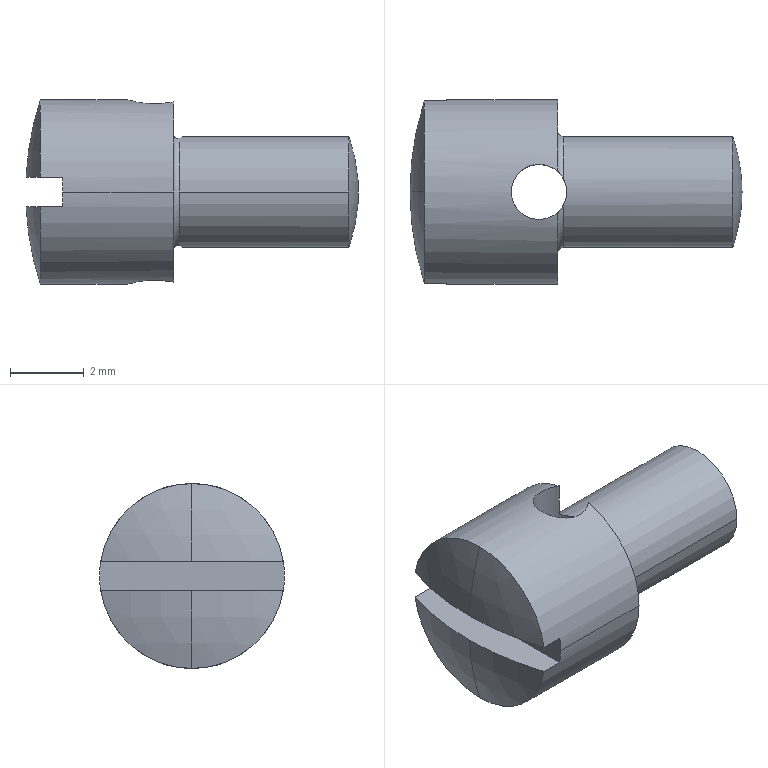Part | NX | features BREP 1 | 1 solid | 19 faces | box 8.99 x 5 x 5 mm | volume 97.359 mm3 | cylinder 6 | sphere 6 | plane 5 | torus 2 | commonest cylinder face diameters 1.5 x2 3 x2 5 x2
STEP:
#1=CARTESIAN_POINT('',(-3.,2.5,0.));
#2=VERTEX_POINT('',#1);
#3=CARTESIAN_POINT('',(0.,2.5,0.));
#4=VERTEX_POINT('',#3);
#5=CARTESIAN_POINT('',(-1.8,2.5,0.));
#6=DIRECTION('',(1.,0.,0.));
#7=VECTOR('',#6,1000.);
#8=LINE('',#5,#7);
#9=EDGE_CURVE('',#2,#4,#8,.T.);
#10=ORIENTED_EDGE('',*,*,#9,.F.);
#11=CARTESIAN_POINT('',(-3.,2.468,0.4));
#12=VERTEX_POINT('',#11);
#13=CARTESIAN_POINT('',(-3.,0.,0.));
#14=DIRECTION('',(1.,0.,0.));
#15=DIRECTION('',(0.,1.,0.));
#16=AXIS2_PLACEMENT_3D('',#13,#14,#15);
#17=CIRCLE('',#16,2.5);
#18=EDGE_CURVE('',#2,#12,#17,.T.);
#19=ORIENTED_EDGE('',*,*,#18,.T.);
#20=CARTESIAN_POINT('',(-3.599,2.468,0.4));
#21=VERTEX_POINT('',#20);
#22=CARTESIAN_POINT('',(-3.3,2.468,0.4));
#23=DIRECTION('',(-1.,0.,0.));
#24=VECTOR('',#23,1000.);
#25=LINE('',#22,#24);
#26=EDGE_CURVE('',#12,#21,#25,.T.);
#27=ORIENTED_EDGE('',*,*,#26,.T.);
#28=CARTESIAN_POINT('',(-3.599,0.,2.5));
#29=VERTEX_POINT('',#28);
#30=CARTESIAN_POINT('',(-3.599,0.,0.));
#31=DIRECTION('',(1.,0.,0.));
#32=DIRECTION('',(0.,1.,0.));
#33=AXIS2_PLACEMENT_3D('',#30,#31,#32);
#34=CIRCLE('',#33,2.5);
#35=EDGE_CURVE('',#21,#29,#34,.T.);
#36=ORIENTED_EDGE('',*,*,#35,.T.);
#37=CARTESIAN_POINT('',(-3.599,-2.468,0.4));
#38=VERTEX_POINT('',#37);
#39=CARTESIAN_POINT('',(-3.599,0.,0.));
#40=DIRECTION('',(1.,0.,0.));
#41=DIRECTION('',(0.,1.,0.));
#42=AXIS2_PLACEMENT_3D('',#39,#40,#41);
#43=CIRCLE('',#42,2.5);
#44=EDGE_CURVE('',#29,#38,#43,.T.);
#45=ORIENTED_EDGE('',*,*,#44,.T.);
#46=CARTESIAN_POINT('',(-3.,-2.468,0.4));
#47=VERTEX_POINT('',#46);
#48=CARTESIAN_POINT('',(-3.3,-2.468,0.4));
#49=DIRECTION('',(1.,0.,0.));
#50=VECTOR('',#49,1000.);
#51=LINE('',#48,#50);
#52=EDGE_CURVE('',#38,#47,#51,.T.);
#53=ORIENTED_EDGE('',*,*,#52,.T.);
#54=CARTESIAN_POINT('',(-3.,-2.5,0.));
#55=VERTEX_POINT('',#54);
#56=CARTESIAN_POINT('',(-3.,0.,0.));
#57=DIRECTION('',(1.,0.,0.));
#58=DIRECTION('',(0.,1.,0.));
#59=AXIS2_PLACEMENT_3D('',#56,#57,#58);
#60=CIRCLE('',#59,2.5);
#61=EDGE_CURVE('',#47,#55,#60,.T.);
#62=ORIENTED_EDGE('',*,*,#61,.T.);
#63=CARTESIAN_POINT('',(0.,-2.5,0.));
#64=VERTEX_POINT('',#63);
#65=CARTESIAN_POINT('',(-1.8,-2.5,0.));
#66=DIRECTION('',(-1.,0.,0.));
#67=VECTOR('',#66,1000.);
#68=LINE('',#65,#67);
#69=EDGE_CURVE('',#64,#55,#68,.T.);
#70=ORIENTED_EDGE('',*,*,#69,.F.);
#71=CARTESIAN_POINT('',(0.,-0.559,2.437));
#72=VERTEX_POINT('',#71);
#73=CARTESIAN_POINT('',(0.,0.,0.));
#74=DIRECTION('',(1.,0.,0.));
#75=DIRECTION('',(0.,1.,0.));
#76=AXIS2_PLACEMENT_3D('',#73,#74,#75);
#77=CIRCLE('',#76,2.5);
#78=EDGE_CURVE('',#72,#64,#77,.T.);
#79=ORIENTED_EDGE('',*,*,#78,.F.);
#80=CARTESIAN_POINT('',(-1.25,0.,2.5));
#81=VERTEX_POINT('',#80);
#82=CARTESIAN_POINT('',(0.,-0.559,2.437));
#83=CARTESIAN_POINT('',(-0.215,-0.7513,2.393));
#84=CARTESIAN_POINT('',(-0.8817,-0.8468,2.363));
#85=CARTESIAN_POINT('',(-1.25,-0.2921,2.5));
#86=CARTESIAN_POINT('',(-1.25,0.,2.5));
#87=B_SPLINE_CURVE_WITH_KNOTS('',3,(#82,#83,#84,#85,#86),.UNSPECIFIED.,.F.,.F.,(4,1,4),(0.,0.0008635,0.001727),.UNSPECIFIED.);
#88=EDGE_CURVE('',#72,#81,#87,.T.);
#89=ORIENTED_EDGE('',*,*,#88,.T.);
#90=CARTESIAN_POINT('',(0.,0.559,2.437));
#91=VERTEX_POINT('',#90);
#92=CARTESIAN_POINT('',(-1.25,0.,2.5));
#93=CARTESIAN_POINT('',(-1.25,0.292,2.5));
#94=CARTESIAN_POINT('',(-0.882,0.8466,2.363));
#95=CARTESIAN_POINT('',(-0.2151,0.7514,2.393));
#96=CARTESIAN_POINT('',(0.,0.559,2.437));
#97=B_SPLINE_CURVE_WITH_KNOTS('',3,(#92,#93,#94,#95,#96),.UNSPECIFIED.,.F.,.F.,(4,1,4),(0.,0.0008633,0.001727),.UNSPECIFIED.);
#98=EDGE_CURVE('',#81,#91,#97,.T.);
#99=ORIENTED_EDGE('',*,*,#98,.T.);
#100=CARTESIAN_POINT('',(0.,0.,0.));
#101=DIRECTION('',(1.,0.,0.));
#102=DIRECTION('',(0.,1.,0.));
#103=AXIS2_PLACEMENT_3D('',#100,#101,#102);
#104=CIRCLE('',#103,2.5);
#105=EDGE_CURVE('',#4,#91,#104,.T.);
#106=ORIENTED_EDGE('',*,*,#105,.F.);
#107=EDGE_LOOP('',(#10,#19,#27,#36,#45,#53,#62,#70,#79,#89,#99,#106));
#108=FACE_BOUND('',#107,.T.);
#109=CARTESIAN_POINT('',(-1.8,0.,0.));
#110=DIRECTION('',(1.,0.,0.));
#111=DIRECTION('',(0.,-1.,0.));
#112=AXIS2_PLACEMENT_3D('',#109,#110,#111);
#113=CYLINDRICAL_SURFACE('',#112,2.5);
#114=ADVANCED_FACE('',(#108),#113,.T.);
#115=CARTESIAN_POINT('',(4.743,0.,-1.5));
#116=VERTEX_POINT('',#115);
#117=CARTESIAN_POINT('',(4.743,0.,1.5));
#118=VERTEX_POINT('',#117);
#119=CARTESIAN_POINT('',(0.5,0.,0.));
#120=DIRECTION('',(0.,-1.,0.));
#121=DIRECTION('',(0.,0.,1.));
#122=AXIS2_PLACEMENT_3D('',#119,#120,#121);
#123=CIRCLE('',#122,4.5);
#124=EDGE_CURVE('',#116,#118,#123,.T.);
#125=ORIENTED_EDGE('',*,*,#124,.F.);
#126=CARTESIAN_POINT('',(4.743,1.5,0.));
#127=VERTEX_POINT('',#126);
#128=CARTESIAN_POINT('',(4.743,0.,0.));
#129=DIRECTION('',(1.,0.,0.));
#130=DIRECTION('',(0.,1.,0.));
#131=AXIS2_PLACEMENT_3D('',#128,#129,#130);
#132=CIRCLE('',#131,1.5);
#133=EDGE_CURVE('',#116,#127,#132,.T.);
#134=ORIENTED_EDGE('',*,*,#133,.T.);
#135=CARTESIAN_POINT('',(4.743,0.,0.));
#136=DIRECTION('',(1.,0.,0.));
#137=DIRECTION('',(0.,1.,0.));
#138=AXIS2_PLACEMENT_3D('',#135,#136,#137);
#139=CIRCLE('',#138,1.5);
#140=EDGE_CURVE('',#127,#118,#139,.T.);
#141=ORIENTED_EDGE('',*,*,#140,.T.);
#142=EDGE_LOOP('',(#125,#134,#141));
#143=FACE_BOUND('',#142,.T.);
#144=CARTESIAN_POINT('',(0.5,0.,0.));
#145=DIRECTION('',(0.,0.,1.));
#146=DIRECTION('',(-1.,0.,0.));
#147=AXIS2_PLACEMENT_3D('',#144,#145,#146);
#148=SPHERICAL_SURFACE('',#147,4.5);
#149=ADVANCED_FACE('',(#143),#148,.T.);
#150=CARTESIAN_POINT('',(-3.99,0.,0.4));
#151=VERTEX_POINT('',#150);
#152=CARTESIAN_POINT('',(4.,0.,0.));
#153=DIRECTION('',(0.,-1.,0.));
#154=DIRECTION('',(0.,0.,1.));
#155=AXIS2_PLACEMENT_3D('',#152,#153,#154);
#156=CIRCLE('',#155,8.);
#157=EDGE_CURVE('',#29,#151,#156,.T.);
#158=ORIENTED_EDGE('',*,*,#157,.F.);
#159=ORIENTED_EDGE('',*,*,#35,.F.);
#160=CARTESIAN_POINT('',(4.,0.,0.4));
#161=DIRECTION('',(0.,0.,1.));
#162=DIRECTION('',(0.,1.,0.));
#163=AXIS2_PLACEMENT_3D('',#160,#161,#162);
#164=CIRCLE('',#163,7.99);
#165=EDGE_CURVE('',#21,#151,#164,.T.);
#166=ORIENTED_EDGE('',*,*,#165,.T.);
#167=EDGE_LOOP('',(#158,#159,#166));
#168=FACE_BOUND('',#167,.T.);
#169=CARTESIAN_POINT('',(4.,0.,0.));
#170=DIRECTION('',(0.,0.,1.));
#171=DIRECTION('',(-1.,0.,0.));
#172=AXIS2_PLACEMENT_3D('',#169,#170,#171);
#173=SPHERICAL_SURFACE('',#172,8.);
#174=ADVANCED_FACE('',(#168),#173,.T.);
#175=CARTESIAN_POINT('',(-3.99,0.,-0.4));
#176=VERTEX_POINT('',#175);
#177=CARTESIAN_POINT('',(-3.599,0.,-2.5));
#178=VERTEX_POINT('',#177);
#179=CARTESIAN_POINT('',(4.,0.,0.));
#180=DIRECTION('',(0.,-1.,0.));
#181=DIRECTION('',(0.,0.,1.));
#182=AXIS2_PLACEMENT_3D('',#179,#180,#181);
#183=CIRCLE('',#182,8.);
#184=EDGE_CURVE('',#176,#178,#183,.T.);
#185=ORIENTED_EDGE('',*,*,#184,.F.);
#186=CARTESIAN_POINT('',(-3.599,2.468,-0.4));
#187=VERTEX_POINT('',#186);
#188=CARTESIAN_POINT('',(4.,0.,-0.4));
#189=DIRECTION('',(0.,0.,-1.));
#190=DIRECTION('',(0.,-1.,0.));
#191=AXIS2_PLACEMENT_3D('',#188,#189,#190);
#192=CIRCLE('',#191,7.99);
#193=EDGE_CURVE('',#176,#187,#192,.T.);
#194=ORIENTED_EDGE('',*,*,#193,.T.);
#195=CARTESIAN_POINT('',(-3.599,0.,0.));
#196=DIRECTION('',(1.,0.,0.));
#197=DIRECTION('',(0.,1.,0.));
#198=AXIS2_PLACEMENT_3D('',#195,#196,#197);
#199=CIRCLE('',#198,2.5);
#200=EDGE_CURVE('',#178,#187,#199,.T.);
#201=ORIENTED_EDGE('',*,*,#200,.F.);
#202=EDGE_LOOP('',(#185,#194,#201));
#203=FACE_BOUND('',#202,.T.);
#204=CARTESIAN_POINT('',(4.,0.,0.));
#205=DIRECTION('',(0.,0.,1.));
#206=DIRECTION('',(-1.,0.,0.));
#207=AXIS2_PLACEMENT_3D('',#204,#205,#206);
#208=SPHERICAL_SURFACE('',#207,8.);
#209=ADVANCED_FACE('',(#203),#208,.T.);
#210=CARTESIAN_POINT('',(0.1624,1.5,0.));
#211=VERTEX_POINT('',#210);
#212=CARTESIAN_POINT('',(2.453,1.5,0.));
#213=DIRECTION('',(1.,0.,0.));
#214=VECTOR('',#213,1000.);
#215=LINE('',#212,#214);
#216=EDGE_CURVE('',#211,#127,#215,.T.);
#217=ORIENTED_EDGE('',*,*,#216,.F.);
#218=CARTESIAN_POINT('',(0.1624,0.3518,1.458));
#219=VERTEX_POINT('',#218);
#220=CARTESIAN_POINT('',(0.1624,0.,0.));
#221=DIRECTION('',(1.,0.,0.));
#222=DIRECTION('',(0.,1.,0.));
#223=AXIS2_PLACEMENT_3D('',#220,#221,#222);
#224=CIRCLE('',#223,1.5);
#225=EDGE_CURVE('',#211,#219,#224,.T.);
#226=ORIENTED_EDGE('',*,*,#225,.T.);
#227=CARTESIAN_POINT('',(0.25,0.,1.5));
#228=VERTEX_POINT('',#227);
#229=CARTESIAN_POINT('',(0.1624,0.3518,1.458));
#230=CARTESIAN_POINT('',(0.2192,0.2448,1.484));
#231=CARTESIAN_POINT('',(0.25,0.124,1.5));
#232=CARTESIAN_POINT('',(0.25,0.,1.5));
#233=B_SPLINE_CURVE_WITH_KNOTS('',3,(#229,#230,#231,#232),.UNSPECIFIED.,.F.,.F.,(4,4),(0.,0.0003667),.UNSPECIFIED.);
#234=EDGE_CURVE('',#219,#228,#233,.T.);
#235=ORIENTED_EDGE('',*,*,#234,.T.);
#236=CARTESIAN_POINT('',(0.1624,-0.3518,1.458));
#237=VERTEX_POINT('',#236);
#238=CARTESIAN_POINT('',(0.25,0.,1.5));
#239=CARTESIAN_POINT('',(0.25,-0.124,1.5));
#240=CARTESIAN_POINT('',(0.2192,-0.2447,1.484));
#241=CARTESIAN_POINT('',(0.1624,-0.3518,1.458));
#242=B_SPLINE_CURVE_WITH_KNOTS('',3,(#238,#239,#240,#241),.UNSPECIFIED.,.F.,.F.,(4,4),(0.,0.0003665),.UNSPECIFIED.);
#243=EDGE_CURVE('',#228,#237,#242,.T.);
#244=ORIENTED_EDGE('',*,*,#243,.T.);
#245=CARTESIAN_POINT('',(0.1624,-1.5,0.));
#246=VERTEX_POINT('',#245);
#247=CARTESIAN_POINT('',(0.1624,0.,0.));
#248=DIRECTION('',(1.,0.,0.));
#249=DIRECTION('',(0.,1.,0.));
#250=AXIS2_PLACEMENT_3D('',#247,#248,#249);
#251=CIRCLE('',#250,1.5);
#252=EDGE_CURVE('',#237,#246,#251,.T.);
#253=ORIENTED_EDGE('',*,*,#252,.T.);
#254=CARTESIAN_POINT('',(4.743,-1.5,0.));
#255=VERTEX_POINT('',#254);
#256=CARTESIAN_POINT('',(2.453,-1.5,0.));
#257=DIRECTION('',(-1.,0.,0.));
#258=VECTOR('',#257,1000.);
#259=LINE('',#256,#258);
#260=EDGE_CURVE('',#255,#246,#259,.T.);
#261=ORIENTED_EDGE('',*,*,#260,.F.);
#262=CARTESIAN_POINT('',(4.743,0.,0.));
#263=DIRECTION('',(1.,0.,0.));
#264=DIRECTION('',(0.,1.,0.));
#265=AXIS2_PLACEMENT_3D('',#262,#263,#264);
#266=CIRCLE('',#265,1.5);
#267=EDGE_CURVE('',#118,#255,#266,.T.);
#268=ORIENTED_EDGE('',*,*,#267,.F.);
#269=ORIENTED_EDGE('',*,*,#140,.F.);
#270=EDGE_LOOP('',(#217,#226,#235,#244,#253,#261,#268,#269));
#271=FACE_BOUND('',#270,.T.);
#272=CARTESIAN_POINT('',(2.453,0.,0.));
#273=DIRECTION('',(1.,0.,0.));
#274=DIRECTION('',(0.,-1.,0.));
#275=AXIS2_PLACEMENT_3D('',#272,#273,#274);
#276=CYLINDRICAL_SURFACE('',#275,1.5);
#277=ADVANCED_FACE('',(#271),#276,.T.);
#278=CARTESIAN_POINT('',(0.25,0.,-1.5));
#279=VERTEX_POINT('',#278);
#280=CARTESIAN_POINT('',(0.25,0.,0.));
#281=DIRECTION('',(0.,0.,-1.));
#282=VECTOR('',#281,1000.);
#283=LINE('',#280,#282);
#284=EDGE_CURVE('',#228,#279,#283,.T.);
#285=ORIENTED_EDGE('',*,*,#284,.F.);
#286=ORIENTED_EDGE('',*,*,#234,.F.);
#287=CARTESIAN_POINT('',(0.,0.559,1.566));
#288=VERTEX_POINT('',#287);
#289=CARTESIAN_POINT('',(0.,0.559,1.566));
#290=CARTESIAN_POINT('',(0.,0.559,1.453));
#291=CARTESIAN_POINT('',(0.1113,0.4479,1.435));
#292=CARTESIAN_POINT('',(0.1624,0.3518,1.458));
#293=B_SPLINE_CURVE_WITH_KNOTS('',3,(#289,#290,#291,#292),.UNSPECIFIED.,.F.,.F.,(4,4),(0.,0.0003331),.UNSPECIFIED.);
#294=EDGE_CURVE('',#288,#219,#293,.T.);
#295=ORIENTED_EDGE('',*,*,#294,.F.);
#296=CARTESIAN_POINT('',(0.,0.559,0.));
#297=DIRECTION('',(0.,0.,-1.));
#298=VECTOR('',#297,1000.);
#299=LINE('',#296,#298);
#300=EDGE_CURVE('',#91,#288,#299,.T.);
#301=ORIENTED_EDGE('',*,*,#300,.F.);
#302=ORIENTED_EDGE('',*,*,#98,.F.);
#303=CARTESIAN_POINT('',(-1.25,0.,-2.5));
#304=VERTEX_POINT('',#303);
#305=CARTESIAN_POINT('',(-1.25,0.,0.));
#306=DIRECTION('',(0.,0.,1.));
#307=VECTOR('',#306,1000.);
#308=LINE('',#305,#307);
#309=EDGE_CURVE('',#304,#81,#308,.T.);
#310=ORIENTED_EDGE('',*,*,#309,.F.);
#311=CARTESIAN_POINT('',(0.,0.559,-2.437));
#312=VERTEX_POINT('',#311);
#313=CARTESIAN_POINT('',(0.,0.559,-2.437));
#314=CARTESIAN_POINT('',(-0.215,0.7513,-2.393));
#315=CARTESIAN_POINT('',(-0.8817,0.8468,-2.363));
#316=CARTESIAN_POINT('',(-1.25,0.2921,-2.5));
#317=CARTESIAN_POINT('',(-1.25,0.,-2.5));
#318=B_SPLINE_CURVE_WITH_KNOTS('',3,(#313,#314,#315,#316,#317),.UNSPECIFIED.,.F.,.F.,(4,1,4),(0.,0.0008635,0.001727),.UNSPECIFIED.);
#319=EDGE_CURVE('',#312,#304,#318,.T.);
#320=ORIENTED_EDGE('',*,*,#319,.F.);
#321=CARTESIAN_POINT('',(0.,0.559,-1.566));
#322=VERTEX_POINT('',#321);
#323=CARTESIAN_POINT('',(0.,0.559,0.));
#324=DIRECTION('',(0.,0.,-1.));
#325=VECTOR('',#324,1000.);
#326=LINE('',#323,#325);
#327=EDGE_CURVE('',#322,#312,#326,.T.);
#328=ORIENTED_EDGE('',*,*,#327,.F.);
#329=CARTESIAN_POINT('',(0.1624,0.3518,-1.458));
#330=VERTEX_POINT('',#329);
#331=CARTESIAN_POINT('',(0.1624,0.3518,-1.458));
#332=CARTESIAN_POINT('',(0.1464,0.3819,-1.451));
#333=CARTESIAN_POINT('',(0.1296,0.4086,-1.446));
#334=CARTESIAN_POINT('',(0.0958,0.4565,-1.443));
#335=CARTESIAN_POINT('',(0.07987,0.4762,-1.445));
#336=CARTESIAN_POINT('',(0.055,0.5047,-1.455));
#337=CARTESIAN_POINT('',(0.04446,0.516,-1.461));
#338=CARTESIAN_POINT('',(0.02656,0.5342,-1.479));
#339=CARTESIAN_POINT('',(0.01932,0.5412,-1.489));
#340=CARTESIAN_POINT('',(0.007644,0.5521,-1.513));
#341=CARTESIAN_POINT('',(0.003645,0.5557,-1.527));
#342=CARTESIAN_POINT('',(-0.0008785,0.5598,-1.56));
#343=CARTESIAN_POINT('',(-0.0003757,0.5594,-1.578));
#344=CARTESIAN_POINT('',(0.005894,0.5537,-1.618));
#345=CARTESIAN_POINT('',(0.01314,0.5472,-1.641));
#346=CARTESIAN_POINT('',(0.02374,0.5368,-1.662));
#347=B_SPLINE_CURVE_WITH_KNOTS('',3,(#331,#332,#333,#334,#335,#336,#337,#338,#339,#340,#341,#342,#343,#344,#345,#346),.UNSPECIFIED.,.F.,.F.,(4,2,2,2,2,2,2,4),(0.,0.169,0.3392,0.466,0.5754,0.6889,0.8273,1.),.UNSPECIFIED.);
#348=EDGE_CURVE('',#330,#322,#347,.T.);
#349=ORIENTED_EDGE('',*,*,#348,.F.);
#350=CARTESIAN_POINT('',(0.25,0.,-1.5));
#351=CARTESIAN_POINT('',(0.25,0.124,-1.5));
#352=CARTESIAN_POINT('',(0.2192,0.2447,-1.484));
#353=CARTESIAN_POINT('',(0.1624,0.3518,-1.458));
#354=B_SPLINE_CURVE_WITH_KNOTS('',3,(#350,#351,#352,#353),.UNSPECIFIED.,.F.,.F.,(4,4),(0.,0.0003665),.UNSPECIFIED.);
#355=EDGE_CURVE('',#279,#330,#354,.T.);
#356=ORIENTED_EDGE('',*,*,#355,.F.);
#357=EDGE_LOOP('',(#285,#286,#295,#301,#302,#310,#320,#328,#349,#356));
#358=FACE_BOUND('',#357,.T.);
#359=CARTESIAN_POINT('',(-0.5,0.,0.));
#360=DIRECTION('',(0.,0.,1.));
#361=DIRECTION('',(-1.,0.,0.));
#362=AXIS2_PLACEMENT_3D('',#359,#360,#361);
#363=CYLINDRICAL_SURFACE('',#362,0.75);
#364=ADVANCED_FACE('',(#358),#363,.F.);
#365=ORIENTED_EDGE('',*,*,#284,.T.);
#366=CARTESIAN_POINT('',(0.1624,-0.3518,-1.458));
#367=VERTEX_POINT('',#366);
#368=CARTESIAN_POINT('',(0.1624,-0.3518,-1.458));
#369=CARTESIAN_POINT('',(0.2192,-0.2448,-1.484));
#370=CARTESIAN_POINT('',(0.25,-0.124,-1.5));
#371=CARTESIAN_POINT('',(0.25,0.,-1.5));
#372=B_SPLINE_CURVE_WITH_KNOTS('',3,(#368,#369,#370,#371),.UNSPECIFIED.,.F.,.F.,(4,4),(0.,0.0003667),.UNSPECIFIED.);
#373=EDGE_CURVE('',#367,#279,#372,.T.);
#374=ORIENTED_EDGE('',*,*,#373,.F.);
#375=CARTESIAN_POINT('',(0.,-0.559,-1.566));
#376=VERTEX_POINT('',#375);
#377=CARTESIAN_POINT('',(0.,-0.559,-1.566));
#378=CARTESIAN_POINT('',(0.,-0.559,-1.453));
#379=CARTESIAN_POINT('',(0.1113,-0.4479,-1.435));
#380=CARTESIAN_POINT('',(0.1624,-0.3518,-1.458));
#381=B_SPLINE_CURVE_WITH_KNOTS('',3,(#377,#378,#379,#380),.UNSPECIFIED.,.F.,.F.,(4,4),(0.,0.0003331),.UNSPECIFIED.);
#382=EDGE_CURVE('',#376,#367,#381,.T.);
#383=ORIENTED_EDGE('',*,*,#382,.F.);
#384=CARTESIAN_POINT('',(0.,-0.559,-2.437));
#385=VERTEX_POINT('',#384);
#386=CARTESIAN_POINT('',(0.,-0.559,0.));
#387=DIRECTION('',(0.,0.,1.));
#388=VECTOR('',#387,1000.);
#389=LINE('',#386,#388);
#390=EDGE_CURVE('',#385,#376,#389,.T.);
#391=ORIENTED_EDGE('',*,*,#390,.F.);
#392=CARTESIAN_POINT('',(-1.25,0.,-2.5));
#393=CARTESIAN_POINT('',(-1.25,-0.292,-2.5));
#394=CARTESIAN_POINT('',(-0.882,-0.8466,-2.363));
#395=CARTESIAN_POINT('',(-0.2151,-0.7514,-2.393));
#396=CARTESIAN_POINT('',(0.,-0.559,-2.437));
#397=B_SPLINE_CURVE_WITH_KNOTS('',3,(#392,#393,#394,#395,#396),.UNSPECIFIED.,.F.,.F.,(4,1,4),(0.,0.0008633,0.001727),.UNSPECIFIED.);
#398=EDGE_CURVE('',#304,#385,#397,.T.);
#399=ORIENTED_EDGE('',*,*,#398,.F.);
#400=ORIENTED_EDGE('',*,*,#309,.T.);
#401=ORIENTED_EDGE('',*,*,#88,.F.);
#402=CARTESIAN_POINT('',(0.,-0.559,1.566));
#403=VERTEX_POINT('',#402);
#404=CARTESIAN_POINT('',(0.,-0.559,0.));
#405=DIRECTION('',(0.,0.,1.));
#406=VECTOR('',#405,1000.);
#407=LINE('',#404,#406);
#408=EDGE_CURVE('',#403,#72,#407,.T.);
#409=ORIENTED_EDGE('',*,*,#408,.F.);
#410=CARTESIAN_POINT('',(0.1624,-0.3518,1.458));
#411=CARTESIAN_POINT('',(0.1464,-0.3819,1.451));
#412=CARTESIAN_POINT('',(0.1296,-0.4086,1.446));
#413=CARTESIAN_POINT('',(0.0958,-0.4565,1.443));
#414=CARTESIAN_POINT('',(0.07987,-0.4762,1.445));
#415=CARTESIAN_POINT('',(0.055,-0.5047,1.455));
#416=CARTESIAN_POINT('',(0.04446,-0.516,1.461));
#417=CARTESIAN_POINT('',(0.02656,-0.5342,1.479));
#418=CARTESIAN_POINT('',(0.01932,-0.5412,1.489));
#419=CARTESIAN_POINT('',(0.007644,-0.5521,1.513));
#420=CARTESIAN_POINT('',(0.003645,-0.5557,1.527));
#421=CARTESIAN_POINT('',(-0.0008785,-0.5598,1.56));
#422=CARTESIAN_POINT('',(-0.0003757,-0.5594,1.578));
#423=CARTESIAN_POINT('',(0.005894,-0.5537,1.618));
#424=CARTESIAN_POINT('',(0.01314,-0.5472,1.641));
#425=CARTESIAN_POINT('',(0.02374,-0.5368,1.662));
#426=B_SPLINE_CURVE_WITH_KNOTS('',3,(#410,#411,#412,#413,#414,#415,#416,#417,#418,#419,#420,#421,#422,#423,#424,#425),.UNSPECIFIED.,.F.,.F.,(4,2,2,2,2,2,2,4),(0.,0.169,0.3392,0.466,0.5754,0.6889,0.8273,1.),.UNSPECIFIED.);
#427=EDGE_CURVE('',#237,#403,#426,.T.);
#428=ORIENTED_EDGE('',*,*,#427,.F.);
#429=ORIENTED_EDGE('',*,*,#243,.F.);
#430=EDGE_LOOP('',(#365,#374,#383,#391,#399,#400,#401,#409,#428,#429));
#431=FACE_BOUND('',#430,.T.);
#432=CARTESIAN_POINT('',(-0.5,0.,0.));
#433=DIRECTION('',(0.,0.,1.));
#434=DIRECTION('',(-1.,0.,0.));
#435=AXIS2_PLACEMENT_3D('',#432,#433,#434);
#436=CYLINDRICAL_SURFACE('',#435,0.75);
#437=ADVANCED_FACE('',(#431),#436,.F.);
#438=ORIENTED_EDGE('',*,*,#216,.T.);
#439=ORIENTED_EDGE('',*,*,#133,.F.);
#440=CARTESIAN_POINT('',(4.743,0.,0.));
#441=DIRECTION('',(1.,0.,0.));
#442=DIRECTION('',(0.,1.,0.));
#443=AXIS2_PLACEMENT_3D('',#440,#441,#442);
#444=CIRCLE('',#443,1.5);
#445=EDGE_CURVE('',#255,#116,#444,.T.);
#446=ORIENTED_EDGE('',*,*,#445,.F.);
#447=ORIENTED_EDGE('',*,*,#260,.T.);
#448=CARTESIAN_POINT('',(0.1624,0.,0.));
#449=DIRECTION('',(1.,0.,0.));
#450=DIRECTION('',(0.,1.,0.));
#451=AXIS2_PLACEMENT_3D('',#448,#449,#450);
#452=CIRCLE('',#451,1.5);
#453=EDGE_CURVE('',#246,#367,#452,.T.);
#454=ORIENTED_EDGE('',*,*,#453,.T.);
#455=ORIENTED_EDGE('',*,*,#373,.T.);
#456=ORIENTED_EDGE('',*,*,#355,.T.);
#457=CARTESIAN_POINT('',(0.1624,0.,0.));
#458=DIRECTION('',(1.,0.,0.));
#459=DIRECTION('',(0.,1.,0.));
#460=AXIS2_PLACEMENT_3D('',#457,#458,#459);
#461=CIRCLE('',#460,1.5);
#462=EDGE_CURVE('',#330,#211,#461,.T.);
#463=ORIENTED_EDGE('',*,*,#462,.T.);
#464=EDGE_LOOP('',(#438,#439,#446,#447,#454,#455,#456,#463));
#465=FACE_BOUND('',#464,.T.);
#466=CARTESIAN_POINT('',(2.453,0.,0.));
#467=DIRECTION('',(1.,0.,0.));
#468=DIRECTION('',(0.,-1.,0.));
#469=AXIS2_PLACEMENT_3D('',#466,#467,#468);
#470=CYLINDRICAL_SURFACE('',#469,1.5);
#471=ADVANCED_FACE('',(#465),#470,.T.);
#472=ORIENTED_EDGE('',*,*,#427,.T.);
#473=CARTESIAN_POINT('',(0.,0.,0.));
#474=DIRECTION('',(1.,0.,0.));
#475=DIRECTION('',(0.,1.,0.));
#476=AXIS2_PLACEMENT_3D('',#473,#474,#475);
#477=CIRCLE('',#476,1.662);
#478=EDGE_CURVE('',#403,#376,#477,.T.);
#479=ORIENTED_EDGE('',*,*,#478,.T.);
#480=ORIENTED_EDGE('',*,*,#382,.T.);
#481=ORIENTED_EDGE('',*,*,#453,.F.);
#482=ORIENTED_EDGE('',*,*,#252,.F.);
#483=EDGE_LOOP('',(#472,#479,#480,#481,#482));
#484=FACE_BOUND('',#483,.T.);
#485=CARTESIAN_POINT('',(0.1624,0.,0.));
#486=DIRECTION('',(1.,0.,0.));
#487=DIRECTION('',(0.,0.,1.));
#488=AXIS2_PLACEMENT_3D('',#485,#486,#487);
#489=TOROIDAL_SURFACE('',#488,1.662,0.1624);
#490=ADVANCED_FACE('',(#484),#489,.F.);
#491=ORIENTED_EDGE('',*,*,#408,.T.);
#492=ORIENTED_EDGE('',*,*,#78,.T.);
#493=CARTESIAN_POINT('',(0.,0.,0.));
#494=DIRECTION('',(1.,0.,0.));
#495=DIRECTION('',(0.,1.,0.));
#496=AXIS2_PLACEMENT_3D('',#493,#494,#495);
#497=CIRCLE('',#496,2.5);
#498=EDGE_CURVE('',#64,#385,#497,.T.);
#499=ORIENTED_EDGE('',*,*,#498,.T.);
#500=ORIENTED_EDGE('',*,*,#390,.T.);
#501=ORIENTED_EDGE('',*,*,#478,.F.);
#502=EDGE_LOOP('',(#491,#492,#499,#500,#501));
#503=FACE_BOUND('',#502,.T.);
#504=CARTESIAN_POINT('',(0.,2.081,0.));
#505=DIRECTION('',(1.,0.,0.));
#506=DIRECTION('',(0.,-1.,0.));
#507=AXIS2_PLACEMENT_3D('',#504,#505,#506);
#508=PLANE('',#507);
#509=ADVANCED_FACE('',(#503),#508,.T.);
#510=ORIENTED_EDGE('',*,*,#26,.F.);
#511=CARTESIAN_POINT('',(-3.,0.,0.4));
#512=DIRECTION('',(0.,1.,0.));
#513=VECTOR('',#512,1000.);
#514=LINE('',#511,#513);
#515=EDGE_CURVE('',#47,#12,#514,.T.);
#516=ORIENTED_EDGE('',*,*,#515,.F.);
#517=ORIENTED_EDGE('',*,*,#52,.F.);
#518=CARTESIAN_POINT('',(4.,0.,0.4));
#519=DIRECTION('',(0.,0.,1.));
#520=DIRECTION('',(0.,1.,0.));
#521=AXIS2_PLACEMENT_3D('',#518,#519,#520);
#522=CIRCLE('',#521,7.99);
#523=EDGE_CURVE('',#151,#38,#522,.T.);
#524=ORIENTED_EDGE('',*,*,#523,.F.);
#525=ORIENTED_EDGE('',*,*,#165,.F.);
#526=EDGE_LOOP('',(#510,#516,#517,#524,#525));
#527=FACE_BOUND('',#526,.T.);
#528=CARTESIAN_POINT('',(-3.55,0.,0.4));
#529=DIRECTION('',(0.,0.,1.));
#530=DIRECTION('',(-1.,0.,0.));
#531=AXIS2_PLACEMENT_3D('',#528,#529,#530);
#532=PLANE('',#531);
#533=ADVANCED_FACE('',(#527),#532,.F.);
#534=CARTESIAN_POINT('',(-3.,2.468,-0.4));
#535=VERTEX_POINT('',#534);
#536=CARTESIAN_POINT('',(-3.3,2.468,-0.4));
#537=DIRECTION('',(1.,0.,0.));
#538=VECTOR('',#537,1000.);
#539=LINE('',#536,#538);
#540=EDGE_CURVE('',#187,#535,#539,.T.);
#541=ORIENTED_EDGE('',*,*,#540,.F.);
#542=ORIENTED_EDGE('',*,*,#193,.F.);
#543=CARTESIAN_POINT('',(-3.599,-2.468,-0.4));
#544=VERTEX_POINT('',#543);
#545=CARTESIAN_POINT('',(4.,0.,-0.4));
#546=DIRECTION('',(0.,0.,-1.));
#547=DIRECTION('',(0.,-1.,0.));
#548=AXIS2_PLACEMENT_3D('',#545,#546,#547);
#549=CIRCLE('',#548,7.99);
#550=EDGE_CURVE('',#544,#176,#549,.T.);
#551=ORIENTED_EDGE('',*,*,#550,.F.);
#552=CARTESIAN_POINT('',(-3.,-2.468,-0.4));
#553=VERTEX_POINT('',#552);
#554=CARTESIAN_POINT('',(-3.3,-2.468,-0.4));
#555=DIRECTION('',(-1.,0.,0.));
#556=VECTOR('',#555,1000.);
#557=LINE('',#554,#556);
#558=EDGE_CURVE('',#553,#544,#557,.T.);
#559=ORIENTED_EDGE('',*,*,#558,.F.);
#560=CARTESIAN_POINT('',(-3.,0.,-0.4));
#561=DIRECTION('',(0.,-1.,0.));
#562=VECTOR('',#561,1000.);
#563=LINE('',#560,#562);
#564=EDGE_CURVE('',#535,#553,#563,.T.);
#565=ORIENTED_EDGE('',*,*,#564,.F.);
#566=EDGE_LOOP('',(#541,#542,#551,#559,#565));
#567=FACE_BOUND('',#566,.T.);
#568=CARTESIAN_POINT('',(-3.55,0.,-0.4));
#569=DIRECTION('',(0.,0.,1.));
#570=DIRECTION('',(-1.,0.,0.));
#571=AXIS2_PLACEMENT_3D('',#568,#569,#570);
#572=PLANE('',#571);
#573=ADVANCED_FACE('',(#567),#572,.T.);
#574=CARTESIAN_POINT('',(-3.,0.,0.));
#575=DIRECTION('',(1.,0.,0.));
#576=DIRECTION('',(0.,1.,0.));
#577=AXIS2_PLACEMENT_3D('',#574,#575,#576);
#578=CIRCLE('',#577,2.5);
#579=EDGE_CURVE('',#535,#2,#578,.T.);
#580=ORIENTED_EDGE('',*,*,#579,.F.);
#581=ORIENTED_EDGE('',*,*,#564,.T.);
#582=CARTESIAN_POINT('',(-3.,0.,0.));
#583=DIRECTION('',(1.,0.,0.));
#584=DIRECTION('',(0.,1.,0.));
#585=AXIS2_PLACEMENT_3D('',#582,#583,#584);
#586=CIRCLE('',#585,2.5);
#587=EDGE_CURVE('',#55,#553,#586,.T.);
#588=ORIENTED_EDGE('',*,*,#587,.F.);
#589=ORIENTED_EDGE('',*,*,#61,.F.);
#590=ORIENTED_EDGE('',*,*,#515,.T.);
#591=ORIENTED_EDGE('',*,*,#18,.F.);
#592=EDGE_LOOP('',(#580,#581,#588,#589,#590,#591));
#593=FACE_BOUND('',#592,.T.);
#594=CARTESIAN_POINT('',(-3.,0.,0.));
#595=DIRECTION('',(-1.,0.,0.));
#596=DIRECTION('',(0.,0.,-1.));
#597=AXIS2_PLACEMENT_3D('',#594,#595,#596);
#598=PLANE('',#597);
#599=ADVANCED_FACE('',(#593),#598,.T.);
#600=ORIENTED_EDGE('',*,*,#184,.T.);
#601=CARTESIAN_POINT('',(-3.599,0.,0.));
#602=DIRECTION('',(1.,0.,0.));
#603=DIRECTION('',(0.,1.,0.));
#604=AXIS2_PLACEMENT_3D('',#601,#602,#603);
#605=CIRCLE('',#604,2.5);
#606=EDGE_CURVE('',#544,#178,#605,.T.);
#607=ORIENTED_EDGE('',*,*,#606,.F.);
#608=ORIENTED_EDGE('',*,*,#550,.T.);
#609=EDGE_LOOP('',(#600,#607,#608));
#610=FACE_BOUND('',#609,.T.);
#611=CARTESIAN_POINT('',(4.,0.,0.));
#612=DIRECTION('',(0.,0.,1.));
#613=DIRECTION('',(-1.,0.,0.));
#614=AXIS2_PLACEMENT_3D('',#611,#612,#613);
#615=SPHERICAL_SURFACE('',#614,8.);
#616=ADVANCED_FACE('',(#610),#615,.T.);
#617=ORIENTED_EDGE('',*,*,#157,.T.);
#618=ORIENTED_EDGE('',*,*,#523,.T.);
#619=ORIENTED_EDGE('',*,*,#44,.F.);
#620=EDGE_LOOP('',(#617,#618,#619));
#621=FACE_BOUND('',#620,.T.);
#622=CARTESIAN_POINT('',(4.,0.,0.));
#623=DIRECTION('',(0.,0.,1.));
#624=DIRECTION('',(-1.,0.,0.));
#625=AXIS2_PLACEMENT_3D('',#622,#623,#624);
#626=SPHERICAL_SURFACE('',#625,8.);
#627=ADVANCED_FACE('',(#621),#626,.T.);
#628=ORIENTED_EDGE('',*,*,#294,.T.);
#629=ORIENTED_EDGE('',*,*,#225,.F.);
#630=ORIENTED_EDGE('',*,*,#462,.F.);
#631=ORIENTED_EDGE('',*,*,#348,.T.);
#632=CARTESIAN_POINT('',(0.,0.,0.));
#633=DIRECTION('',(1.,0.,0.));
#634=DIRECTION('',(0.,1.,0.));
#635=AXIS2_PLACEMENT_3D('',#632,#633,#634);
#636=CIRCLE('',#635,1.662);
#637=EDGE_CURVE('',#322,#288,#636,.T.);
#638=ORIENTED_EDGE('',*,*,#637,.T.);
#639=EDGE_LOOP('',(#628,#629,#630,#631,#638));
#640=FACE_BOUND('',#639,.T.);
#641=CARTESIAN_POINT('',(0.1624,0.,0.));
#642=DIRECTION('',(1.,0.,0.));
#643=DIRECTION('',(0.,0.,1.));
#644=AXIS2_PLACEMENT_3D('',#641,#642,#643);
#645=TOROIDAL_SURFACE('',#644,1.662,0.1624);
#646=ADVANCED_FACE('',(#640),#645,.F.);
#647=ORIENTED_EDGE('',*,*,#124,.T.);
#648=ORIENTED_EDGE('',*,*,#267,.T.);
#649=ORIENTED_EDGE('',*,*,#445,.T.);
#650=EDGE_LOOP('',(#647,#648,#649));
#651=FACE_BOUND('',#650,.T.);
#652=CARTESIAN_POINT('',(0.5,0.,0.));
#653=DIRECTION('',(0.,0.,1.));
#654=DIRECTION('',(-1.,0.,0.));
#655=AXIS2_PLACEMENT_3D('',#652,#653,#654);
#656=SPHERICAL_SURFACE('',#655,4.5);
#657=ADVANCED_FACE('',(#651),#656,.T.);
#658=ORIENTED_EDGE('',*,*,#9,.T.);
#659=CARTESIAN_POINT('',(0.,0.,0.));
#660=DIRECTION('',(1.,0.,0.));
#661=DIRECTION('',(0.,1.,0.));
#662=AXIS2_PLACEMENT_3D('',#659,#660,#661);
#663=CIRCLE('',#662,2.5);
#664=EDGE_CURVE('',#312,#4,#663,.T.);
#665=ORIENTED_EDGE('',*,*,#664,.F.);
#666=ORIENTED_EDGE('',*,*,#319,.T.);
#667=ORIENTED_EDGE('',*,*,#398,.T.);
#668=ORIENTED_EDGE('',*,*,#498,.F.);
#669=ORIENTED_EDGE('',*,*,#69,.T.);
#670=ORIENTED_EDGE('',*,*,#587,.T.);
#671=ORIENTED_EDGE('',*,*,#558,.T.);
#672=ORIENTED_EDGE('',*,*,#606,.T.);
#673=ORIENTED_EDGE('',*,*,#200,.T.);
#674=ORIENTED_EDGE('',*,*,#540,.T.);
#675=ORIENTED_EDGE('',*,*,#579,.T.);
#676=EDGE_LOOP('',(#658,#665,#666,#667,#668,#669,#670,#671,#672,#673,#674,#675));
#677=FACE_BOUND('',#676,.T.);
#678=CARTESIAN_POINT('',(-1.8,0.,0.));
#679=DIRECTION('',(1.,0.,0.));
#680=DIRECTION('',(0.,-1.,0.));
#681=AXIS2_PLACEMENT_3D('',#678,#679,#680);
#682=CYLINDRICAL_SURFACE('',#681,2.5);
#683=ADVANCED_FACE('',(#677),#682,.T.);
#684=ORIENTED_EDGE('',*,*,#300,.T.);
#685=ORIENTED_EDGE('',*,*,#637,.F.);
#686=ORIENTED_EDGE('',*,*,#327,.T.);
#687=ORIENTED_EDGE('',*,*,#664,.T.);
#688=ORIENTED_EDGE('',*,*,#105,.T.);
#689=EDGE_LOOP('',(#684,#685,#686,#687,#688));
#690=FACE_BOUND('',#689,.T.);
#691=CARTESIAN_POINT('',(0.,2.081,0.));
#692=DIRECTION('',(1.,0.,0.));
#693=DIRECTION('',(0.,-1.,0.));
#694=AXIS2_PLACEMENT_3D('',#691,#692,#693);
#695=PLANE('',#694);
#696=ADVANCED_FACE('',(#690),#695,.T.);
#697=CLOSED_SHELL('',(#114,#149,#174,#209,#277,#364,#437,#471,#490,#509,#533,#573,#599,#616,#627,#646,#657,#683,#696));
#698=MANIFOLD_SOLID_BREP('',#697);
#699=(LENGTH_UNIT()NAMED_UNIT(*)SI_UNIT(.MILLI.,.METRE.));
#700=UNCERTAINTY_MEASURE_WITH_UNIT(LENGTH_MEASURE(0.0508),#699,'','');
#701=(NAMED_UNIT(*)PLANE_ANGLE_UNIT()SI_UNIT($,.RADIAN.));
#702=(NAMED_UNIT(*)SI_UNIT($,.STERADIAN.)SOLID_ANGLE_UNIT());
#703=(GEOMETRIC_REPRESENTATION_CONTEXT(3)GLOBAL_UNCERTAINTY_ASSIGNED_CONTEXT((#700))GLOBAL_UNIT_ASSIGNED_CONTEXT((#699,#701,#702))REPRESENTATION_CONTEXT('',''));
#704=ADVANCED_BREP_SHAPE_REPRESENTATION('',(#698),#703);